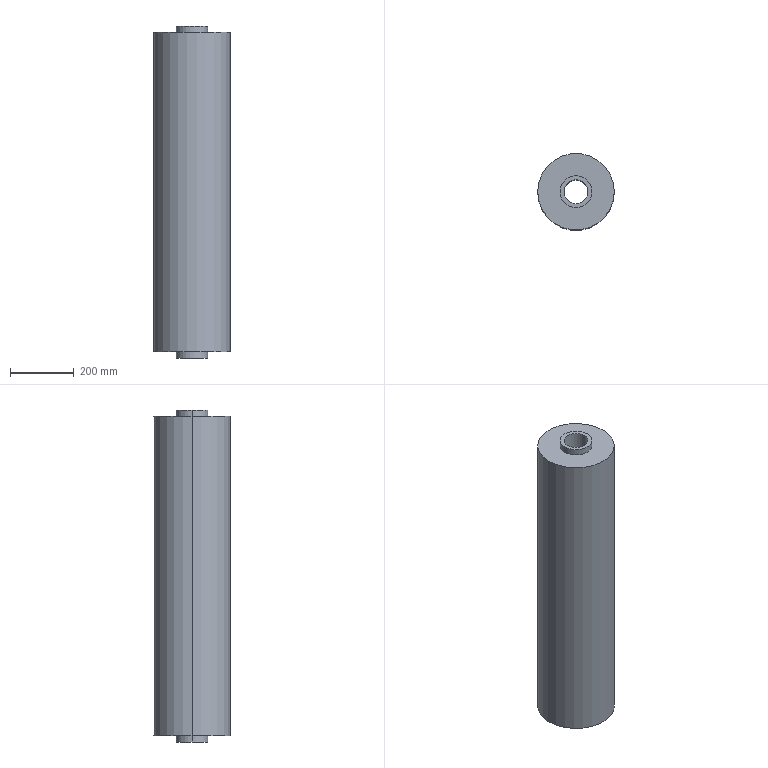Part | SolidWorks | features ICE 2, Extrusion 1, MirrorPattern 1 | 1 solid | 12 faces | box 240 x 240 x 1040 mm | volume 40958514 mm3 | cylinder 8 | plane 4 | commonest cylinder face diameters 100 x4 75 x2 240 x2
STEP:
#1=CARTESIAN_POINT('',(50.,0.,-20.));
#2=VERTEX_POINT('',#1);
#3=CARTESIAN_POINT('',(-50.,0.,-20.));
#4=VERTEX_POINT('',#3);
#5=CARTESIAN_POINT('',(0.,0.,-20.));
#6=DIRECTION('',(0.,0.,1.));
#7=DIRECTION('',(1.,0.,0.));
#8=AXIS2_PLACEMENT_3D('',#5,#6,#7);
#9=CIRCLE('',#8,50.);
#10=EDGE_CURVE('',#2,#4,#9,.T.);
#11=ORIENTED_EDGE('',*,*,#10,.T.);
#12=CARTESIAN_POINT('',(-50.,0.,0.));
#13=VERTEX_POINT('',#12);
#14=CARTESIAN_POINT('',(-50.,0.,-20.));
#15=DIRECTION('',(0.,0.,1.));
#16=VECTOR('',#15,1000.);
#17=LINE('',#14,#16);
#18=EDGE_CURVE('',#4,#13,#17,.T.);
#19=ORIENTED_EDGE('',*,*,#18,.T.);
#20=CARTESIAN_POINT('',(50.,0.,0.));
#21=VERTEX_POINT('',#20);
#22=CARTESIAN_POINT('',(0.,0.,0.));
#23=DIRECTION('',(0.,0.,1.));
#24=DIRECTION('',(1.,0.,0.));
#25=AXIS2_PLACEMENT_3D('',#22,#23,#24);
#26=CIRCLE('',#25,50.);
#27=EDGE_CURVE('',#21,#13,#26,.T.);
#28=ORIENTED_EDGE('',*,*,#27,.F.);
#29=CARTESIAN_POINT('',(50.,0.,-20.));
#30=DIRECTION('',(0.,0.,1.));
#31=VECTOR('',#30,1000.);
#32=LINE('',#29,#31);
#33=EDGE_CURVE('',#2,#21,#32,.T.);
#34=ORIENTED_EDGE('',*,*,#33,.F.);
#35=EDGE_LOOP('',(#11,#19,#28,#34));
#36=FACE_OUTER_BOUND('',#35,.T.);
#37=CARTESIAN_POINT('',(0.,0.,-20.));
#38=DIRECTION('',(0.,0.,1.));
#39=DIRECTION('',(1.,0.,0.));
#40=AXIS2_PLACEMENT_3D('',#37,#38,#39);
#41=CYLINDRICAL_SURFACE('',#40,50.);
#42=ADVANCED_FACE('',(#36),#41,.T.);
#43=CARTESIAN_POINT('',(50.,0.,1020.));
#44=VERTEX_POINT('',#43);
#45=CARTESIAN_POINT('',(-50.,0.,1020.));
#46=VERTEX_POINT('',#45);
#47=CARTESIAN_POINT('',(0.,0.,1020.));
#48=DIRECTION('',(0.,0.,1.));
#49=DIRECTION('',(1.,0.,0.));
#50=AXIS2_PLACEMENT_3D('',#47,#48,#49);
#51=CIRCLE('',#50,50.);
#52=EDGE_CURVE('',#44,#46,#51,.T.);
#53=ORIENTED_EDGE('',*,*,#52,.F.);
#54=CARTESIAN_POINT('',(50.,0.,1000.));
#55=VERTEX_POINT('',#54);
#56=CARTESIAN_POINT('',(50.,0.,1020.));
#57=DIRECTION('',(0.,0.,-1.));
#58=VECTOR('',#57,1000.);
#59=LINE('',#56,#58);
#60=EDGE_CURVE('',#44,#55,#59,.T.);
#61=ORIENTED_EDGE('',*,*,#60,.T.);
#62=CARTESIAN_POINT('',(-50.,0.,1000.));
#63=VERTEX_POINT('',#62);
#64=CARTESIAN_POINT('',(0.,0.,1000.));
#65=DIRECTION('',(0.,0.,1.));
#66=DIRECTION('',(1.,0.,0.));
#67=AXIS2_PLACEMENT_3D('',#64,#65,#66);
#68=CIRCLE('',#67,50.);
#69=EDGE_CURVE('',#55,#63,#68,.T.);
#70=ORIENTED_EDGE('',*,*,#69,.T.);
#71=CARTESIAN_POINT('',(-50.,0.,1020.));
#72=DIRECTION('',(0.,0.,-1.));
#73=VECTOR('',#72,1000.);
#74=LINE('',#71,#73);
#75=EDGE_CURVE('',#46,#63,#74,.T.);
#76=ORIENTED_EDGE('',*,*,#75,.F.);
#77=EDGE_LOOP('',(#53,#61,#70,#76));
#78=FACE_OUTER_BOUND('',#77,.T.);
#79=CARTESIAN_POINT('',(0.,0.,1020.));
#80=DIRECTION('',(0.,0.,-1.));
#81=DIRECTION('',(-1.,0.,0.));
#82=AXIS2_PLACEMENT_3D('',#79,#80,#81);
#83=CYLINDRICAL_SURFACE('',#82,50.);
#84=ADVANCED_FACE('',(#78),#83,.T.);
#85=CARTESIAN_POINT('',(-37.5,0.,-20.));
#86=VERTEX_POINT('',#85);
#87=CARTESIAN_POINT('',(37.5,0.,-20.));
#88=VERTEX_POINT('',#87);
#89=CARTESIAN_POINT('',(0.,0.,-20.));
#90=DIRECTION('',(0.,0.,1.));
#91=DIRECTION('',(1.,0.,0.));
#92=AXIS2_PLACEMENT_3D('',#89,#90,#91);
#93=CIRCLE('',#92,37.5);
#94=EDGE_CURVE('',#86,#88,#93,.T.);
#95=ORIENTED_EDGE('',*,*,#94,.F.);
#96=CARTESIAN_POINT('',(-37.5,0.,1020.));
#97=VERTEX_POINT('',#96);
#98=CARTESIAN_POINT('',(-37.5,0.,0.));
#99=DIRECTION('',(0.,0.,1.));
#100=VECTOR('',#99,1000.);
#101=LINE('',#98,#100);
#102=EDGE_CURVE('',#86,#97,#101,.T.);
#103=ORIENTED_EDGE('',*,*,#102,.T.);
#104=CARTESIAN_POINT('',(37.5,0.,1020.));
#105=VERTEX_POINT('',#104);
#106=CARTESIAN_POINT('',(0.,0.,1020.));
#107=DIRECTION('',(0.,0.,1.));
#108=DIRECTION('',(1.,0.,0.));
#109=AXIS2_PLACEMENT_3D('',#106,#107,#108);
#110=CIRCLE('',#109,37.5);
#111=EDGE_CURVE('',#97,#105,#110,.T.);
#112=ORIENTED_EDGE('',*,*,#111,.T.);
#113=CARTESIAN_POINT('',(37.5,0.,0.));
#114=DIRECTION('',(0.,0.,1.));
#115=VECTOR('',#114,1000.);
#116=LINE('',#113,#115);
#117=EDGE_CURVE('',#88,#105,#116,.T.);
#118=ORIENTED_EDGE('',*,*,#117,.F.);
#119=EDGE_LOOP('',(#95,#103,#112,#118));
#120=FACE_OUTER_BOUND('',#119,.T.);
#121=CARTESIAN_POINT('',(0.,0.,0.));
#122=DIRECTION('',(0.,0.,1.));
#123=DIRECTION('',(1.,0.,0.));
#124=AXIS2_PLACEMENT_3D('',#121,#122,#123);
#125=CYLINDRICAL_SURFACE('',#124,37.5);
#126=ADVANCED_FACE('',(#120),#125,.F.);
#127=CARTESIAN_POINT('',(120.,0.,1000.));
#128=VERTEX_POINT('',#127);
#129=CARTESIAN_POINT('',(-120.,0.,1000.));
#130=VERTEX_POINT('',#129);
#131=CARTESIAN_POINT('',(0.,0.,1000.));
#132=DIRECTION('',(0.,0.,1.));
#133=DIRECTION('',(1.,0.,0.));
#134=AXIS2_PLACEMENT_3D('',#131,#132,#133);
#135=CIRCLE('',#134,120.);
#136=EDGE_CURVE('',#128,#130,#135,.T.);
#137=ORIENTED_EDGE('',*,*,#136,.F.);
#138=CARTESIAN_POINT('',(120.,0.,0.));
#139=VERTEX_POINT('',#138);
#140=CARTESIAN_POINT('',(120.,0.,1000.));
#141=DIRECTION('',(0.,0.,-1.));
#142=VECTOR('',#141,1000.);
#143=LINE('',#140,#142);
#144=EDGE_CURVE('',#128,#139,#143,.T.);
#145=ORIENTED_EDGE('',*,*,#144,.T.);
#146=CARTESIAN_POINT('',(-120.,0.,0.));
#147=VERTEX_POINT('',#146);
#148=CARTESIAN_POINT('',(0.,0.,0.));
#149=DIRECTION('',(0.,0.,1.));
#150=DIRECTION('',(1.,0.,0.));
#151=AXIS2_PLACEMENT_3D('',#148,#149,#150);
#152=CIRCLE('',#151,120.);
#153=EDGE_CURVE('',#139,#147,#152,.T.);
#154=ORIENTED_EDGE('',*,*,#153,.T.);
#155=CARTESIAN_POINT('',(-120.,0.,1000.));
#156=DIRECTION('',(0.,0.,-1.));
#157=VECTOR('',#156,1000.);
#158=LINE('',#155,#157);
#159=EDGE_CURVE('',#130,#147,#158,.T.);
#160=ORIENTED_EDGE('',*,*,#159,.F.);
#161=EDGE_LOOP('',(#137,#145,#154,#160));
#162=FACE_OUTER_BOUND('',#161,.T.);
#163=CARTESIAN_POINT('',(0.,0.,1000.));
#164=DIRECTION('',(0.,0.,-1.));
#165=DIRECTION('',(-1.,0.,0.));
#166=AXIS2_PLACEMENT_3D('',#163,#164,#165);
#167=CYLINDRICAL_SURFACE('',#166,120.);
#168=ADVANCED_FACE('',(#162),#167,.T.);
#169=CARTESIAN_POINT('',(0.,0.,1000.));
#170=DIRECTION('',(0.,0.,1.));
#171=DIRECTION('',(1.,0.,0.));
#172=AXIS2_PLACEMENT_3D('',#169,#170,#171);
#173=CIRCLE('',#172,120.);
#174=EDGE_CURVE('',#130,#128,#173,.T.);
#175=ORIENTED_EDGE('',*,*,#174,.T.);
#176=ORIENTED_EDGE('',*,*,#136,.T.);
#177=EDGE_LOOP('',(#175,#176));
#178=FACE_OUTER_BOUND('',#177,.T.);
#179=CARTESIAN_POINT('',(0.,0.,1000.));
#180=DIRECTION('',(0.,0.,1.));
#181=DIRECTION('',(1.,0.,0.));
#182=AXIS2_PLACEMENT_3D('',#179,#180,#181);
#183=CIRCLE('',#182,50.);
#184=EDGE_CURVE('',#63,#55,#183,.T.);
#185=ORIENTED_EDGE('',*,*,#184,.F.);
#186=ORIENTED_EDGE('',*,*,#69,.F.);
#187=EDGE_LOOP('',(#185,#186));
#188=FACE_BOUND('',#187,.T.);
#189=CARTESIAN_POINT('',(0.,0.,1000.));
#190=DIRECTION('',(0.,0.,1.));
#191=DIRECTION('',(1.,0.,0.));
#192=AXIS2_PLACEMENT_3D('',#189,#190,#191);
#193=PLANE('',#192);
#194=ADVANCED_FACE('',(#178,#188),#193,.T.);
#195=ORIENTED_EDGE('',*,*,#144,.F.);
#196=ORIENTED_EDGE('',*,*,#174,.F.);
#197=ORIENTED_EDGE('',*,*,#159,.T.);
#198=CARTESIAN_POINT('',(0.,0.,0.));
#199=DIRECTION('',(0.,0.,1.));
#200=DIRECTION('',(1.,0.,0.));
#201=AXIS2_PLACEMENT_3D('',#198,#199,#200);
#202=CIRCLE('',#201,120.);
#203=EDGE_CURVE('',#147,#139,#202,.T.);
#204=ORIENTED_EDGE('',*,*,#203,.T.);
#205=EDGE_LOOP('',(#195,#196,#197,#204));
#206=FACE_OUTER_BOUND('',#205,.T.);
#207=CARTESIAN_POINT('',(0.,0.,1000.));
#208=DIRECTION('',(0.,0.,-1.));
#209=DIRECTION('',(-1.,0.,0.));
#210=AXIS2_PLACEMENT_3D('',#207,#208,#209);
#211=CYLINDRICAL_SURFACE('',#210,120.);
#212=ADVANCED_FACE('',(#206),#211,.T.);
#213=ORIENTED_EDGE('',*,*,#27,.T.);
#214=CARTESIAN_POINT('',(0.,0.,0.));
#215=DIRECTION('',(0.,0.,1.));
#216=DIRECTION('',(1.,0.,0.));
#217=AXIS2_PLACEMENT_3D('',#214,#215,#216);
#218=CIRCLE('',#217,50.);
#219=EDGE_CURVE('',#13,#21,#218,.T.);
#220=ORIENTED_EDGE('',*,*,#219,.T.);
#221=EDGE_LOOP('',(#213,#220));
#222=FACE_BOUND('',#221,.T.);
#223=ORIENTED_EDGE('',*,*,#203,.F.);
#224=ORIENTED_EDGE('',*,*,#153,.F.);
#225=EDGE_LOOP('',(#223,#224));
#226=FACE_OUTER_BOUND('',#225,.T.);
#227=CARTESIAN_POINT('',(0.,0.,0.));
#228=DIRECTION('',(0.,0.,1.));
#229=DIRECTION('',(1.,0.,0.));
#230=AXIS2_PLACEMENT_3D('',#227,#228,#229);
#231=PLANE('',#230);
#232=ADVANCED_FACE('',(#222,#226),#231,.F.);
#233=ORIENTED_EDGE('',*,*,#102,.F.);
#234=CARTESIAN_POINT('',(0.,0.,-20.));
#235=DIRECTION('',(0.,0.,1.));
#236=DIRECTION('',(1.,0.,0.));
#237=AXIS2_PLACEMENT_3D('',#234,#235,#236);
#238=CIRCLE('',#237,37.5);
#239=EDGE_CURVE('',#88,#86,#238,.T.);
#240=ORIENTED_EDGE('',*,*,#239,.F.);
#241=ORIENTED_EDGE('',*,*,#117,.T.);
#242=CARTESIAN_POINT('',(0.,0.,1020.));
#243=DIRECTION('',(0.,0.,1.));
#244=DIRECTION('',(1.,0.,0.));
#245=AXIS2_PLACEMENT_3D('',#242,#243,#244);
#246=CIRCLE('',#245,37.5);
#247=EDGE_CURVE('',#105,#97,#246,.T.);
#248=ORIENTED_EDGE('',*,*,#247,.T.);
#249=EDGE_LOOP('',(#233,#240,#241,#248));
#250=FACE_OUTER_BOUND('',#249,.T.);
#251=CARTESIAN_POINT('',(0.,0.,0.));
#252=DIRECTION('',(0.,0.,1.));
#253=DIRECTION('',(1.,0.,0.));
#254=AXIS2_PLACEMENT_3D('',#251,#252,#253);
#255=CYLINDRICAL_SURFACE('',#254,37.5);
#256=ADVANCED_FACE('',(#250),#255,.F.);
#257=CARTESIAN_POINT('',(0.,0.,1020.));
#258=DIRECTION('',(0.,0.,1.));
#259=DIRECTION('',(1.,0.,0.));
#260=AXIS2_PLACEMENT_3D('',#257,#258,#259);
#261=CIRCLE('',#260,50.);
#262=EDGE_CURVE('',#46,#44,#261,.T.);
#263=ORIENTED_EDGE('',*,*,#262,.T.);
#264=ORIENTED_EDGE('',*,*,#52,.T.);
#265=EDGE_LOOP('',(#263,#264));
#266=FACE_OUTER_BOUND('',#265,.T.);
#267=ORIENTED_EDGE('',*,*,#247,.F.);
#268=ORIENTED_EDGE('',*,*,#111,.F.);
#269=EDGE_LOOP('',(#267,#268));
#270=FACE_BOUND('',#269,.T.);
#271=CARTESIAN_POINT('',(0.,0.,1020.));
#272=DIRECTION('',(0.,0.,1.));
#273=DIRECTION('',(1.,0.,0.));
#274=AXIS2_PLACEMENT_3D('',#271,#272,#273);
#275=PLANE('',#274);
#276=ADVANCED_FACE('',(#266,#270),#275,.T.);
#277=ORIENTED_EDGE('',*,*,#60,.F.);
#278=ORIENTED_EDGE('',*,*,#262,.F.);
#279=ORIENTED_EDGE('',*,*,#75,.T.);
#280=ORIENTED_EDGE('',*,*,#184,.T.);
#281=EDGE_LOOP('',(#277,#278,#279,#280));
#282=FACE_OUTER_BOUND('',#281,.T.);
#283=CARTESIAN_POINT('',(0.,0.,1020.));
#284=DIRECTION('',(0.,0.,-1.));
#285=DIRECTION('',(-1.,0.,0.));
#286=AXIS2_PLACEMENT_3D('',#283,#284,#285);
#287=CYLINDRICAL_SURFACE('',#286,50.);
#288=ADVANCED_FACE('',(#282),#287,.T.);
#289=ORIENTED_EDGE('',*,*,#18,.F.);
#290=CARTESIAN_POINT('',(0.,0.,-20.));
#291=DIRECTION('',(0.,0.,1.));
#292=DIRECTION('',(1.,0.,0.));
#293=AXIS2_PLACEMENT_3D('',#290,#291,#292);
#294=CIRCLE('',#293,50.);
#295=EDGE_CURVE('',#4,#2,#294,.T.);
#296=ORIENTED_EDGE('',*,*,#295,.T.);
#297=ORIENTED_EDGE('',*,*,#33,.T.);
#298=ORIENTED_EDGE('',*,*,#219,.F.);
#299=EDGE_LOOP('',(#289,#296,#297,#298));
#300=FACE_OUTER_BOUND('',#299,.T.);
#301=CARTESIAN_POINT('',(0.,0.,-20.));
#302=DIRECTION('',(0.,0.,1.));
#303=DIRECTION('',(1.,0.,0.));
#304=AXIS2_PLACEMENT_3D('',#301,#302,#303);
#305=CYLINDRICAL_SURFACE('',#304,50.);
#306=ADVANCED_FACE('',(#300),#305,.T.);
#307=ORIENTED_EDGE('',*,*,#239,.T.);
#308=ORIENTED_EDGE('',*,*,#94,.T.);
#309=EDGE_LOOP('',(#307,#308));
#310=FACE_BOUND('',#309,.T.);
#311=ORIENTED_EDGE('',*,*,#10,.F.);
#312=ORIENTED_EDGE('',*,*,#295,.F.);
#313=EDGE_LOOP('',(#311,#312));
#314=FACE_OUTER_BOUND('',#313,.T.);
#315=CARTESIAN_POINT('',(0.,0.,-20.));
#316=DIRECTION('',(0.,0.,-1.));
#317=DIRECTION('',(1.,0.,0.));
#318=AXIS2_PLACEMENT_3D('',#315,#316,#317);
#319=PLANE('',#318);
#320=ADVANCED_FACE('',(#310,#314),#319,.T.);
#321=CLOSED_SHELL('',(#42,#84,#126,#168,#194,#212,#232,#256,#276,#288,#306,#320));
#322=MANIFOLD_SOLID_BREP('',#321);
#323=CARTESIAN_POINT('',(0.,0.,0.));
#324=DIRECTION('',(0.,0.,1.));
#325=DIRECTION('',(1.,0.,0.));
#326=AXIS2_PLACEMENT_3D('',#323,#324,#325);
#327=(LENGTH_UNIT()NAMED_UNIT(*)SI_UNIT(.MILLI.,.METRE.));
#328=UNCERTAINTY_MEASURE_WITH_UNIT(LENGTH_MEASURE(0.00001),#327,'','');
#329=(NAMED_UNIT(*)PLANE_ANGLE_UNIT()SI_UNIT($,.RADIAN.));
#330=(NAMED_UNIT(*)SI_UNIT($,.STERADIAN.)SOLID_ANGLE_UNIT());
#331=(GEOMETRIC_REPRESENTATION_CONTEXT(3)GLOBAL_UNCERTAINTY_ASSIGNED_CONTEXT((#328))GLOBAL_UNIT_ASSIGNED_CONTEXT((#327,#329,#330))REPRESENTATION_CONTEXT('',''));
#332=ADVANCED_BREP_SHAPE_REPRESENTATION('',(#322,#326),#331);